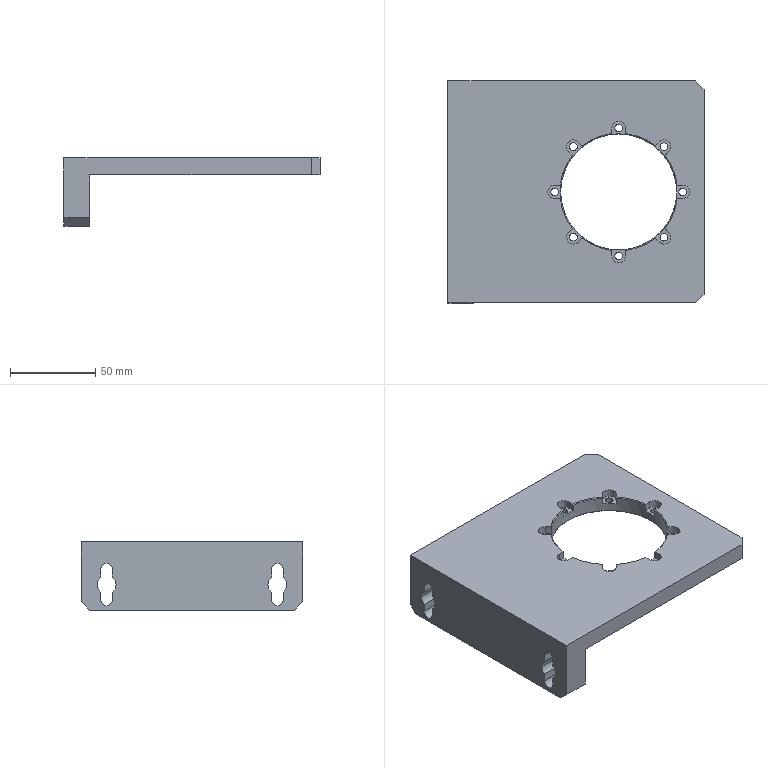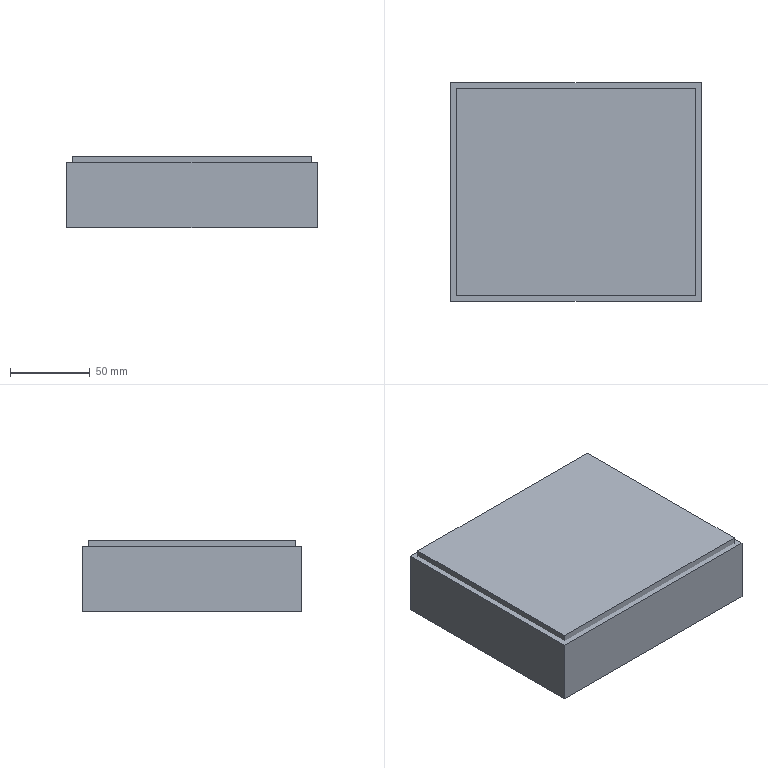CAM job | NX | 3+2 milling, drilling | part box 150 x 130 x 40 mm | stock box 157 x 137 x 45 mm
Tools:
number,name,description,diameter,corner_radius,flute_length,length,flutes
19,D80,Milling Tool-5 Parameters,80.0,0.0,50.0,75.0,2
1,D6A45,Milling Tool-5 Parameters,6.0,0.0,50.0,75.0,2
8,4.5ZT,Drilling Tool,4.5,0.0,35.0,50.0,2
15,D10,Milling Tool-5 Parameters,10.0,0.0,50.0,75.0,2
14,D10JING,Milling Tool-5 Parameters,10.0,0.0,50.0,75.0,2
12,D6,Milling Tool-5 Parameters,6.0,0.0,50.0,75.0,2
11,D4,Milling Tool-5 Parameters,4.0,0.0,50.0,75.0,2
Operations:
program,operation,operation_type,tool,method,geometry_group,spindle_rpm,surface_speed,feed_per_tooth,feed_cut,feed_plunge,cut_length_mm,path_length_mm,cut_time_min,machine_time_min
1,FLOOR_WALL_COPY,VolumeBased25DMillingOperation,D80,METHOD,A,6500.0,1633.0,0.1154,1500.0,100.0,831.997,885.997,0.5547,0.5601
1,DRILLING_COPY_1,Operation,D6A45,METHOD,A,5000.0,94.0,0.035,350.0,0.0,32.0,347.003,0.0914,0.1229
1,DRILLING_COPY_COPY_COPY_2,Operation,4.5ZT,METHOD,A,2000.0,20.0,0.045,180.0,0.0,126.816,536.634,0.7045,0.7455
1,ADAPTIVE_MILLING,CavityMilling,D10,METHOD,A,9500.0,298.0,0.1579,3000.0,1000.0,6257.336,7001.622,2.094,2.168
1,ADAPTIVE_MILLING_COPY,CavityMilling,D10,METHOD,A,9500.0,298.0,0.1579,3000.0,1000.0,6039.511,6103.511,3.006,3.013
1,ZLEVEL_PROFILE_COPY_1_COPY_COPY_1,ZLevelMilling,D10JING,METHOD,A,9500.0,298.0,0.0632,1200.0,1000.0,1185.793,1425.153,0.9893,1.013
1,ZLEVEL_PROFILE,ZLevelMilling,D6,METHOD,A,9500.0,179.0,0.1053,2000.0,100.0,1433.741,2150.591,0.7169,0.7886
1,PLANAR_MILL_COPY_COPY_COPY_COPY_COPY_COPY_1,PlanarMilling,D6A45,METHOD,A,9500.0,179.0,0.0658,1250.0,100.0,876.732,1037.843,0.7014,0.7175
1,刀补14,ZLevelMilling,D10JING,METHOD,A,9500.0,298.0,0.0632,1200.0,1000.0,189.79,267.79,0.1588,0.1666
2,ZLEVEL_PROFILE_1,ZLevelMilling,D4,METHOD,B,9500.0,119.0,0.0737,1400.0,1000.0,3753.436,4000.804,2.702,2.727
2,PLANAR_MILL_COPY_COPY_COPY_COPY_COPY_COPY_1_COPY,PlanarMilling,D6A45,METHOD,B,9500.0,179.0,0.0658,1250.0,100.0,122.725,338.325,0.0982,0.1197
3,FLOOR_WALL_COPY_COPY,VolumeBased25DMillingOperation,D80,METHOD,C,6500.0,1633.0,0.1154,1500.0,100.0,8039.97,10868.098,5.36,5.643
3,FLOOR_WALL,VolumeBased25DMillingOperation,D10,METHOD,C,9500.0,298.0,0.1579,3000.0,1000.0,48406.045,48803.566,16.143,16.183
3,FLOOR_WALL_COPY_1,VolumeBased25DMillingOperation,D10JING,METHOD,C,9500.0,298.0,0.0632,1200.0,1000.0,304.0,647.7,0.2553,0.2897
3,FLOOR_WALL_COPY_1_COPY,VolumeBased25DMillingOperation,D10JING,METHOD,C,9500.0,298.0,0.0632,1200.0,1000.0,4164.537,4393.037,3.472,3.495
3,PLANAR_MILL_COPY_COPY_COPY_COPY_COPY_COPY_1_COPY_COPY,PlanarMilling,D6A45,METHOD,C,9500.0,179.0,0.0658,1250.0,100.0,302.194,361.194,0.2418,0.2477
3,PLANAR_MILL_COPY_COPY_COPY_COPY_COPY_COPY_1_COPY_COPY_COPY,PlanarMilling,D6A45,METHOD,C,9500.0,179.0,0.0658,1250.0,100.0,736.923,2368.743,0.5895,0.7527
3,ZLEVEL_PROFILE_1_COPY,ZLevelMilling,D6A45,METHOD,C,9500.0,179.0,0.0737,1400.0,1000.0,983.34,1234.478,0.705,0.7301